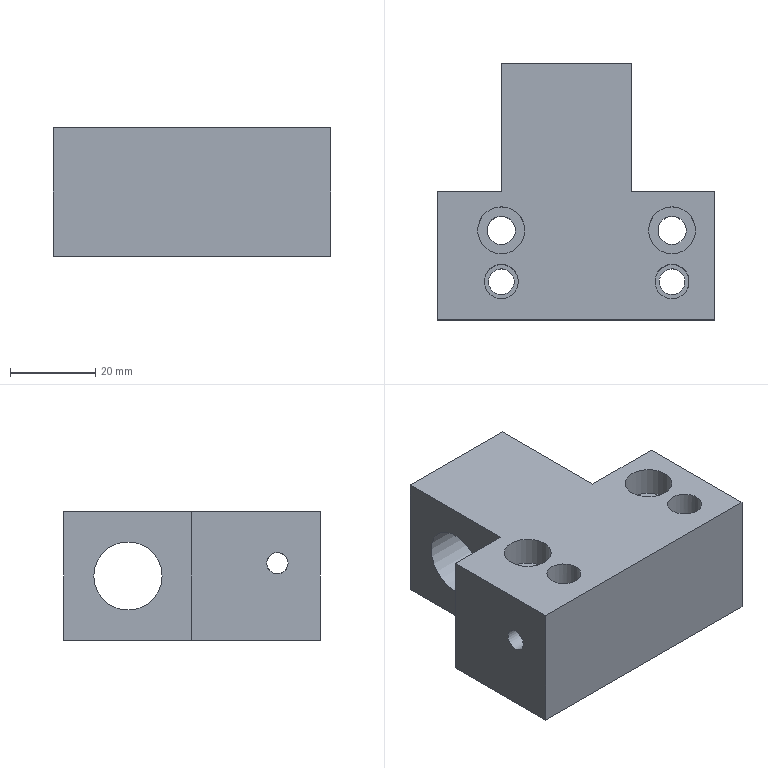Part | NX | features 5003_228_Bracket 2 | 1 solid | 26 faces | box 65 x 60 x 30 mm | volume 73363 mm3 | plane 14 | cylinder 12 | commonest cylinder face diameters 5 x3 6 x2 6.6 x2 8 x2 11 x2 16 x1
STEP:
#1=CARTESIAN_POINT('',(44.6,-182.,-208.));
#2=VERTEX_POINT('',#1);
#3=CARTESIAN_POINT('',(109.6,-182.,-208.));
#4=VERTEX_POINT('',#3);
#5=CARTESIAN_POINT('',(44.6,-182.,-208.));
#6=DIRECTION('',(1.,0.,0.));
#7=VECTOR('',#6,1000.);
#8=LINE('',#5,#7);
#9=EDGE_CURVE('',#2,#4,#8,.T.);
#10=ORIENTED_EDGE('',*,*,#9,.F.);
#11=CARTESIAN_POINT('',(44.6,-182.,-238.));
#12=VERTEX_POINT('',#11);
#13=CARTESIAN_POINT('',(44.6,-182.,-238.));
#14=DIRECTION('',(0.,0.,1.));
#15=VECTOR('',#14,1000.);
#16=LINE('',#13,#15);
#17=EDGE_CURVE('',#12,#2,#16,.T.);
#18=ORIENTED_EDGE('',*,*,#17,.F.);
#19=CARTESIAN_POINT('',(109.6,-182.,-238.));
#20=VERTEX_POINT('',#19);
#21=CARTESIAN_POINT('',(44.6,-182.,-238.));
#22=DIRECTION('',(1.,0.,0.));
#23=VECTOR('',#22,1000.);
#24=LINE('',#21,#23);
#25=EDGE_CURVE('',#12,#20,#24,.T.);
#26=ORIENTED_EDGE('',*,*,#25,.T.);
#27=CARTESIAN_POINT('',(109.6,-182.,-238.));
#28=DIRECTION('',(0.,0.,1.));
#29=VECTOR('',#28,1000.);
#30=LINE('',#27,#29);
#31=EDGE_CURVE('',#20,#4,#30,.T.);
#32=ORIENTED_EDGE('',*,*,#31,.T.);
#33=EDGE_LOOP('',(#10,#18,#26,#32));
#34=FACE_BOUND('',#33,.T.);
#35=CARTESIAN_POINT('',(44.6,-182.,-238.));
#36=DIRECTION('',(0.,-1.,0.));
#37=DIRECTION('',(1.,0.,0.));
#38=AXIS2_PLACEMENT_3D('',#35,#36,#37);
#39=PLANE('',#38);
#40=ADVANCED_FACE('',(#34),#39,.T.);
#41=CARTESIAN_POINT('',(44.6,-174.5,-220.));
#42=VERTEX_POINT('',#41);
#43=CARTESIAN_POINT('',(44.6,-172.,-220.));
#44=DIRECTION('',(-1.,0.,0.));
#45=DIRECTION('',(0.,-1.,0.));
#46=AXIS2_PLACEMENT_3D('',#43,#44,#45);
#47=CIRCLE('',#46,2.5);
#48=EDGE_CURVE('',#42,#42,#47,.T.);
#49=ORIENTED_EDGE('',*,*,#48,.F.);
#50=EDGE_LOOP('',(#49));
#51=FACE_BOUND('',#50,.T.);
#52=CARTESIAN_POINT('',(44.6,-152.,-208.));
#53=VERTEX_POINT('',#52);
#54=CARTESIAN_POINT('',(44.6,-152.,-238.));
#55=VERTEX_POINT('',#54);
#56=CARTESIAN_POINT('',(44.6,-152.,-208.));
#57=DIRECTION('',(0.,0.,-1.));
#58=VECTOR('',#57,1000.);
#59=LINE('',#56,#58);
#60=EDGE_CURVE('',#53,#55,#59,.T.);
#61=ORIENTED_EDGE('',*,*,#60,.T.);
#62=CARTESIAN_POINT('',(44.6,-122.,-238.));
#63=DIRECTION('',(0.,-1.,0.));
#64=VECTOR('',#63,1000.);
#65=LINE('',#62,#64);
#66=EDGE_CURVE('',#55,#12,#65,.T.);
#67=ORIENTED_EDGE('',*,*,#66,.T.);
#68=ORIENTED_EDGE('',*,*,#17,.T.);
#69=CARTESIAN_POINT('',(44.6,-122.,-208.));
#70=DIRECTION('',(0.,-1.,0.));
#71=VECTOR('',#70,1000.);
#72=LINE('',#69,#71);
#73=EDGE_CURVE('',#53,#2,#72,.T.);
#74=ORIENTED_EDGE('',*,*,#73,.F.);
#75=EDGE_LOOP('',(#61,#67,#68,#74));
#76=FACE_BOUND('',#75,.T.);
#77=CARTESIAN_POINT('',(44.6,-122.,-238.));
#78=DIRECTION('',(-1.,0.,0.));
#79=DIRECTION('',(0.,-1.,0.));
#80=AXIS2_PLACEMENT_3D('',#77,#78,#79);
#81=PLANE('',#80);
#82=ADVANCED_FACE('',(#51,#76),#81,.T.);
#83=CARTESIAN_POINT('',(90.089,-122.,-208.));
#84=VERTEX_POINT('',#83);
#85=CARTESIAN_POINT('',(90.089,-122.,-238.));
#86=VERTEX_POINT('',#85);
#87=CARTESIAN_POINT('',(90.089,-122.,-208.));
#88=DIRECTION('',(0.,0.,-1.));
#89=VECTOR('',#88,1000.);
#90=LINE('',#87,#89);
#91=EDGE_CURVE('',#84,#86,#90,.T.);
#92=ORIENTED_EDGE('',*,*,#91,.T.);
#93=CARTESIAN_POINT('',(59.6,-122.,-238.));
#94=VERTEX_POINT('',#93);
#95=CARTESIAN_POINT('',(109.6,-122.,-238.));
#96=DIRECTION('',(-1.,0.,0.));
#97=VECTOR('',#96,1000.);
#98=LINE('',#95,#97);
#99=EDGE_CURVE('',#86,#94,#98,.T.);
#100=ORIENTED_EDGE('',*,*,#99,.T.);
#101=CARTESIAN_POINT('',(59.6,-122.,-208.));
#102=VERTEX_POINT('',#101);
#103=CARTESIAN_POINT('',(59.6,-122.,-208.));
#104=DIRECTION('',(0.,0.,-1.));
#105=VECTOR('',#104,1000.);
#106=LINE('',#103,#105);
#107=EDGE_CURVE('',#102,#94,#106,.T.);
#108=ORIENTED_EDGE('',*,*,#107,.F.);
#109=CARTESIAN_POINT('',(109.6,-122.,-208.));
#110=DIRECTION('',(-1.,0.,0.));
#111=VECTOR('',#110,1000.);
#112=LINE('',#109,#111);
#113=EDGE_CURVE('',#84,#102,#112,.T.);
#114=ORIENTED_EDGE('',*,*,#113,.F.);
#115=EDGE_LOOP('',(#92,#100,#108,#114));
#116=FACE_BOUND('',#115,.T.);
#117=CARTESIAN_POINT('',(109.6,-122.,-238.));
#118=DIRECTION('',(0.,1.,0.));
#119=DIRECTION('',(-1.,0.,0.));
#120=AXIS2_PLACEMENT_3D('',#117,#118,#119);
#121=PLANE('',#120);
#122=ADVANCED_FACE('',(#116),#121,.T.);
#123=CARTESIAN_POINT('',(109.6,-169.5,-220.));
#124=VERTEX_POINT('',#123);
#125=CARTESIAN_POINT('',(109.6,-172.,-220.));
#126=DIRECTION('',(1.,0.,0.));
#127=DIRECTION('',(0.,1.,0.));
#128=AXIS2_PLACEMENT_3D('',#125,#126,#127);
#129=CIRCLE('',#128,2.5);
#130=EDGE_CURVE('',#124,#124,#129,.T.);
#131=ORIENTED_EDGE('',*,*,#130,.F.);
#132=EDGE_LOOP('',(#131));
#133=FACE_BOUND('',#132,.T.);
#134=CARTESIAN_POINT('',(109.6,-152.,-208.));
#135=VERTEX_POINT('',#134);
#136=CARTESIAN_POINT('',(109.6,-152.,-238.));
#137=VERTEX_POINT('',#136);
#138=CARTESIAN_POINT('',(109.6,-152.,-208.));
#139=DIRECTION('',(0.,0.,-1.));
#140=VECTOR('',#139,1000.);
#141=LINE('',#138,#140);
#142=EDGE_CURVE('',#135,#137,#141,.T.);
#143=ORIENTED_EDGE('',*,*,#142,.F.);
#144=CARTESIAN_POINT('',(109.6,-182.,-208.));
#145=DIRECTION('',(0.,1.,0.));
#146=VECTOR('',#145,1000.);
#147=LINE('',#144,#146);
#148=EDGE_CURVE('',#4,#135,#147,.T.);
#149=ORIENTED_EDGE('',*,*,#148,.F.);
#150=ORIENTED_EDGE('',*,*,#31,.F.);
#151=CARTESIAN_POINT('',(109.6,-182.,-238.));
#152=DIRECTION('',(0.,1.,0.));
#153=VECTOR('',#152,1000.);
#154=LINE('',#151,#153);
#155=EDGE_CURVE('',#20,#137,#154,.T.);
#156=ORIENTED_EDGE('',*,*,#155,.T.);
#157=EDGE_LOOP('',(#143,#149,#150,#156));
#158=FACE_BOUND('',#157,.T.);
#159=CARTESIAN_POINT('',(109.6,-182.,-238.));
#160=DIRECTION('',(1.,0.,0.));
#161=DIRECTION('',(0.,1.,0.));
#162=AXIS2_PLACEMENT_3D('',#159,#160,#161);
#163=PLANE('',#162);
#164=ADVANCED_FACE('',(#133,#158),#163,.T.);
#165=CARTESIAN_POINT('',(99.6,-176.,-238.));
#166=VERTEX_POINT('',#165);
#167=CARTESIAN_POINT('',(99.6,-173.,-238.));
#168=DIRECTION('',(0.,0.,1.));
#169=DIRECTION('',(0.,-1.,0.));
#170=AXIS2_PLACEMENT_3D('',#167,#168,#169);
#171=CIRCLE('',#170,3.);
#172=EDGE_CURVE('',#166,#166,#171,.T.);
#173=ORIENTED_EDGE('',*,*,#172,.T.);
#174=EDGE_LOOP('',(#173));
#175=FACE_BOUND('',#174,.T.);
#176=CARTESIAN_POINT('',(59.6,-176.,-238.));
#177=VERTEX_POINT('',#176);
#178=CARTESIAN_POINT('',(59.6,-173.,-238.));
#179=DIRECTION('',(0.,0.,1.));
#180=DIRECTION('',(0.,-1.,0.));
#181=AXIS2_PLACEMENT_3D('',#178,#179,#180);
#182=CIRCLE('',#181,3.);
#183=EDGE_CURVE('',#177,#177,#182,.T.);
#184=ORIENTED_EDGE('',*,*,#183,.T.);
#185=EDGE_LOOP('',(#184));
#186=FACE_BOUND('',#185,.T.);
#187=CARTESIAN_POINT('',(59.6,-164.3,-238.));
#188=VERTEX_POINT('',#187);
#189=CARTESIAN_POINT('',(59.6,-161.,-238.));
#190=DIRECTION('',(0.,0.,1.));
#191=DIRECTION('',(0.,-1.,0.));
#192=AXIS2_PLACEMENT_3D('',#189,#190,#191);
#193=CIRCLE('',#192,3.3);
#194=EDGE_CURVE('',#188,#188,#193,.T.);
#195=ORIENTED_EDGE('',*,*,#194,.T.);
#196=EDGE_LOOP('',(#195));
#197=FACE_BOUND('',#196,.T.);
#198=CARTESIAN_POINT('',(99.6,-164.3,-238.));
#199=VERTEX_POINT('',#198);
#200=CARTESIAN_POINT('',(99.6,-161.,-238.));
#201=DIRECTION('',(0.,0.,1.));
#202=DIRECTION('',(0.,-1.,0.));
#203=AXIS2_PLACEMENT_3D('',#200,#201,#202);
#204=CIRCLE('',#203,3.3);
#205=EDGE_CURVE('',#199,#199,#204,.T.);
#206=ORIENTED_EDGE('',*,*,#205,.T.);
#207=EDGE_LOOP('',(#206));
#208=FACE_BOUND('',#207,.T.);
#209=ORIENTED_EDGE('',*,*,#99,.F.);
#210=CARTESIAN_POINT('',(90.089,-152.,-238.));
#211=VERTEX_POINT('',#210);
#212=CARTESIAN_POINT('',(90.089,-152.,-238.));
#213=DIRECTION('',(0.,1.,0.));
#214=VECTOR('',#213,1000.);
#215=LINE('',#212,#214);
#216=EDGE_CURVE('',#211,#86,#215,.T.);
#217=ORIENTED_EDGE('',*,*,#216,.F.);
#218=CARTESIAN_POINT('',(109.6,-152.,-238.));
#219=DIRECTION('',(-1.,0.,0.));
#220=VECTOR('',#219,1000.);
#221=LINE('',#218,#220);
#222=EDGE_CURVE('',#137,#211,#221,.T.);
#223=ORIENTED_EDGE('',*,*,#222,.F.);
#224=ORIENTED_EDGE('',*,*,#155,.F.);
#225=ORIENTED_EDGE('',*,*,#25,.F.);
#226=ORIENTED_EDGE('',*,*,#66,.F.);
#227=CARTESIAN_POINT('',(59.6,-152.,-238.));
#228=VERTEX_POINT('',#227);
#229=CARTESIAN_POINT('',(59.6,-152.,-238.));
#230=DIRECTION('',(-1.,0.,0.));
#231=VECTOR('',#230,1000.);
#232=LINE('',#229,#231);
#233=EDGE_CURVE('',#228,#55,#232,.T.);
#234=ORIENTED_EDGE('',*,*,#233,.F.);
#235=CARTESIAN_POINT('',(59.6,-122.,-238.));
#236=DIRECTION('',(0.,-1.,0.));
#237=VECTOR('',#236,1000.);
#238=LINE('',#235,#237);
#239=EDGE_CURVE('',#94,#228,#238,.T.);
#240=ORIENTED_EDGE('',*,*,#239,.F.);
#241=EDGE_LOOP('',(#209,#217,#223,#224,#225,#226,#234,#240));
#242=FACE_BOUND('',#241,.T.);
#243=CARTESIAN_POINT('',(114.6,-182.,-238.));
#244=DIRECTION('',(0.,0.,1.));
#245=DIRECTION('',(0.,-1.,0.));
#246=AXIS2_PLACEMENT_3D('',#243,#244,#245);
#247=PLANE('',#246);
#248=ADVANCED_FACE('',(#175,#186,#197,#208,#242),#247,.F.);
#249=CARTESIAN_POINT('',(99.6,-177.,-208.));
#250=VERTEX_POINT('',#249);
#251=CARTESIAN_POINT('',(99.6,-173.,-208.));
#252=DIRECTION('',(0.,0.,1.));
#253=DIRECTION('',(0.,-1.,0.));
#254=AXIS2_PLACEMENT_3D('',#251,#252,#253);
#255=CIRCLE('',#254,4.);
#256=EDGE_CURVE('',#250,#250,#255,.T.);
#257=ORIENTED_EDGE('',*,*,#256,.F.);
#258=EDGE_LOOP('',(#257));
#259=FACE_BOUND('',#258,.T.);
#260=CARTESIAN_POINT('',(59.6,-177.,-208.));
#261=VERTEX_POINT('',#260);
#262=CARTESIAN_POINT('',(59.6,-173.,-208.));
#263=DIRECTION('',(0.,0.,1.));
#264=DIRECTION('',(0.,-1.,0.));
#265=AXIS2_PLACEMENT_3D('',#262,#263,#264);
#266=CIRCLE('',#265,4.);
#267=EDGE_CURVE('',#261,#261,#266,.T.);
#268=ORIENTED_EDGE('',*,*,#267,.F.);
#269=EDGE_LOOP('',(#268));
#270=FACE_BOUND('',#269,.T.);
#271=CARTESIAN_POINT('',(59.6,-166.5,-208.));
#272=VERTEX_POINT('',#271);
#273=CARTESIAN_POINT('',(59.6,-161.,-208.));
#274=DIRECTION('',(0.,0.,1.));
#275=DIRECTION('',(0.,-1.,0.));
#276=AXIS2_PLACEMENT_3D('',#273,#274,#275);
#277=CIRCLE('',#276,5.5);
#278=EDGE_CURVE('',#272,#272,#277,.T.);
#279=ORIENTED_EDGE('',*,*,#278,.F.);
#280=EDGE_LOOP('',(#279));
#281=FACE_BOUND('',#280,.T.);
#282=CARTESIAN_POINT('',(99.6,-166.5,-208.));
#283=VERTEX_POINT('',#282);
#284=CARTESIAN_POINT('',(99.6,-161.,-208.));
#285=DIRECTION('',(0.,0.,1.));
#286=DIRECTION('',(0.,-1.,0.));
#287=AXIS2_PLACEMENT_3D('',#284,#285,#286);
#288=CIRCLE('',#287,5.5);
#289=EDGE_CURVE('',#283,#283,#288,.T.);
#290=ORIENTED_EDGE('',*,*,#289,.F.);
#291=EDGE_LOOP('',(#290));
#292=FACE_BOUND('',#291,.T.);
#293=CARTESIAN_POINT('',(90.089,-152.,-208.));
#294=VERTEX_POINT('',#293);
#295=CARTESIAN_POINT('',(90.089,-152.,-208.));
#296=DIRECTION('',(0.,1.,0.));
#297=VECTOR('',#296,1000.);
#298=LINE('',#295,#297);
#299=EDGE_CURVE('',#294,#84,#298,.T.);
#300=ORIENTED_EDGE('',*,*,#299,.T.);
#301=ORIENTED_EDGE('',*,*,#113,.T.);
#302=CARTESIAN_POINT('',(59.6,-152.,-208.));
#303=VERTEX_POINT('',#302);
#304=CARTESIAN_POINT('',(59.6,-122.,-208.));
#305=DIRECTION('',(0.,-1.,0.));
#306=VECTOR('',#305,1000.);
#307=LINE('',#304,#306);
#308=EDGE_CURVE('',#102,#303,#307,.T.);
#309=ORIENTED_EDGE('',*,*,#308,.T.);
#310=CARTESIAN_POINT('',(59.6,-152.,-208.));
#311=DIRECTION('',(-1.,0.,0.));
#312=VECTOR('',#311,1000.);
#313=LINE('',#310,#312);
#314=EDGE_CURVE('',#303,#53,#313,.T.);
#315=ORIENTED_EDGE('',*,*,#314,.T.);
#316=ORIENTED_EDGE('',*,*,#73,.T.);
#317=ORIENTED_EDGE('',*,*,#9,.T.);
#318=ORIENTED_EDGE('',*,*,#148,.T.);
#319=CARTESIAN_POINT('',(109.6,-152.,-208.));
#320=DIRECTION('',(-1.,0.,0.));
#321=VECTOR('',#320,1000.);
#322=LINE('',#319,#321);
#323=EDGE_CURVE('',#135,#294,#322,.T.);
#324=ORIENTED_EDGE('',*,*,#323,.T.);
#325=EDGE_LOOP('',(#300,#301,#309,#315,#316,#317,#318,#324));
#326=FACE_BOUND('',#325,.T.);
#327=CARTESIAN_POINT('',(114.6,-182.,-208.));
#328=DIRECTION('',(0.,0.,1.));
#329=DIRECTION('',(0.,-1.,0.));
#330=AXIS2_PLACEMENT_3D('',#327,#328,#329);
#331=PLANE('',#330);
#332=ADVANCED_FACE('',(#259,#270,#281,#292,#326),#331,.T.);
#333=ORIENTED_EDGE('',*,*,#233,.T.);
#334=ORIENTED_EDGE('',*,*,#60,.F.);
#335=ORIENTED_EDGE('',*,*,#314,.F.);
#336=CARTESIAN_POINT('',(59.6,-152.,-208.));
#337=DIRECTION('',(0.,0.,-1.));
#338=VECTOR('',#337,1000.);
#339=LINE('',#336,#338);
#340=EDGE_CURVE('',#303,#228,#339,.T.);
#341=ORIENTED_EDGE('',*,*,#340,.T.);
#342=EDGE_LOOP('',(#333,#334,#335,#341));
#343=FACE_BOUND('',#342,.T.);
#344=CARTESIAN_POINT('',(59.6,-152.,-208.));
#345=DIRECTION('',(0.,-1.,0.));
#346=DIRECTION('',(1.,0.,0.));
#347=AXIS2_PLACEMENT_3D('',#344,#345,#346);
#348=PLANE('',#347);
#349=ADVANCED_FACE('',(#343),#348,.F.);
#350=CARTESIAN_POINT('',(59.6,-145.,-223.));
#351=VERTEX_POINT('',#350);
#352=CARTESIAN_POINT('',(59.6,-137.,-223.));
#353=DIRECTION('',(-1.,0.,0.));
#354=DIRECTION('',(0.,-1.,0.));
#355=AXIS2_PLACEMENT_3D('',#352,#353,#354);
#356=CIRCLE('',#355,8.);
#357=EDGE_CURVE('',#351,#351,#356,.T.);
#358=ORIENTED_EDGE('',*,*,#357,.F.);
#359=EDGE_LOOP('',(#358));
#360=FACE_BOUND('',#359,.T.);
#361=ORIENTED_EDGE('',*,*,#239,.T.);
#362=ORIENTED_EDGE('',*,*,#340,.F.);
#363=ORIENTED_EDGE('',*,*,#308,.F.);
#364=ORIENTED_EDGE('',*,*,#107,.T.);
#365=EDGE_LOOP('',(#361,#362,#363,#364));
#366=FACE_BOUND('',#365,.T.);
#367=CARTESIAN_POINT('',(59.6,-122.,-208.));
#368=DIRECTION('',(1.,0.,0.));
#369=DIRECTION('',(0.,1.,0.));
#370=AXIS2_PLACEMENT_3D('',#367,#368,#369);
#371=PLANE('',#370);
#372=ADVANCED_FACE('',(#360,#366),#371,.F.);
#373=CARTESIAN_POINT('',(90.089,-145.,-223.));
#374=VERTEX_POINT('',#373);
#375=CARTESIAN_POINT('',(90.089,-137.,-223.));
#376=DIRECTION('',(-1.,0.,0.));
#377=DIRECTION('',(0.,-1.,0.));
#378=AXIS2_PLACEMENT_3D('',#375,#376,#377);
#379=CIRCLE('',#378,8.);
#380=EDGE_CURVE('',#374,#374,#379,.T.);
#381=ORIENTED_EDGE('',*,*,#380,.T.);
#382=EDGE_LOOP('',(#381));
#383=FACE_BOUND('',#382,.T.);
#384=ORIENTED_EDGE('',*,*,#216,.T.);
#385=ORIENTED_EDGE('',*,*,#91,.F.);
#386=ORIENTED_EDGE('',*,*,#299,.F.);
#387=CARTESIAN_POINT('',(90.089,-152.,-208.));
#388=DIRECTION('',(0.,0.,-1.));
#389=VECTOR('',#388,1000.);
#390=LINE('',#387,#389);
#391=EDGE_CURVE('',#294,#211,#390,.T.);
#392=ORIENTED_EDGE('',*,*,#391,.T.);
#393=EDGE_LOOP('',(#384,#385,#386,#392));
#394=FACE_BOUND('',#393,.T.);
#395=CARTESIAN_POINT('',(90.089,-152.,-208.));
#396=DIRECTION('',(-1.,0.,0.));
#397=DIRECTION('',(0.,-1.,0.));
#398=AXIS2_PLACEMENT_3D('',#395,#396,#397);
#399=PLANE('',#398);
#400=ADVANCED_FACE('',(#383,#394),#399,.F.);
#401=ORIENTED_EDGE('',*,*,#222,.T.);
#402=ORIENTED_EDGE('',*,*,#391,.F.);
#403=ORIENTED_EDGE('',*,*,#323,.F.);
#404=ORIENTED_EDGE('',*,*,#142,.T.);
#405=EDGE_LOOP('',(#401,#402,#403,#404));
#406=FACE_BOUND('',#405,.T.);
#407=CARTESIAN_POINT('',(109.6,-152.,-208.));
#408=DIRECTION('',(0.,-1.,0.));
#409=DIRECTION('',(1.,0.,0.));
#410=AXIS2_PLACEMENT_3D('',#407,#408,#409);
#411=PLANE('',#410);
#412=ADVANCED_FACE('',(#406),#411,.F.);
#413=ORIENTED_EDGE('',*,*,#357,.T.);
#414=EDGE_LOOP('',(#413));
#415=FACE_BOUND('',#414,.T.);
#416=ORIENTED_EDGE('',*,*,#380,.F.);
#417=EDGE_LOOP('',(#416));
#418=FACE_BOUND('',#417,.T.);
#419=CARTESIAN_POINT('',(59.6,-137.,-223.));
#420=DIRECTION('',(-1.,0.,0.));
#421=DIRECTION('',(0.,-1.,0.));
#422=AXIS2_PLACEMENT_3D('',#419,#420,#421);
#423=CYLINDRICAL_SURFACE('',#422,8.);
#424=ADVANCED_FACE('',(#415,#418),#423,.F.);
#425=ORIENTED_EDGE('',*,*,#205,.F.);
#426=EDGE_LOOP('',(#425));
#427=FACE_BOUND('',#426,.T.);
#428=CARTESIAN_POINT('',(99.6,-164.3,-214.8));
#429=VERTEX_POINT('',#428);
#430=CARTESIAN_POINT('',(99.6,-161.,-214.8));
#431=DIRECTION('',(0.,0.,1.));
#432=DIRECTION('',(0.,-1.,0.));
#433=AXIS2_PLACEMENT_3D('',#430,#431,#432);
#434=CIRCLE('',#433,3.3);
#435=EDGE_CURVE('',#429,#429,#434,.T.);
#436=ORIENTED_EDGE('',*,*,#435,.T.);
#437=EDGE_LOOP('',(#436));
#438=FACE_BOUND('',#437,.T.);
#439=CARTESIAN_POINT('',(99.6,-161.,-208.));
#440=DIRECTION('',(0.,0.,1.));
#441=DIRECTION('',(0.,-1.,0.));
#442=AXIS2_PLACEMENT_3D('',#439,#440,#441);
#443=CYLINDRICAL_SURFACE('',#442,3.3);
#444=ADVANCED_FACE('',(#427,#438),#443,.F.);
#445=ORIENTED_EDGE('',*,*,#435,.F.);
#446=EDGE_LOOP('',(#445));
#447=FACE_BOUND('',#446,.T.);
#448=CARTESIAN_POINT('',(99.6,-166.5,-214.8));
#449=VERTEX_POINT('',#448);
#450=CARTESIAN_POINT('',(99.6,-161.,-214.8));
#451=DIRECTION('',(0.,0.,1.));
#452=DIRECTION('',(0.,-1.,0.));
#453=AXIS2_PLACEMENT_3D('',#450,#451,#452);
#454=CIRCLE('',#453,5.5);
#455=EDGE_CURVE('',#449,#449,#454,.T.);
#456=ORIENTED_EDGE('',*,*,#455,.T.);
#457=EDGE_LOOP('',(#456));
#458=FACE_BOUND('',#457,.T.);
#459=CARTESIAN_POINT('',(102.9,-161.,-214.8));
#460=DIRECTION('',(0.,0.,-1.));
#461=DIRECTION('',(0.,1.,0.));
#462=AXIS2_PLACEMENT_3D('',#459,#460,#461);
#463=PLANE('',#462);
#464=ADVANCED_FACE('',(#447,#458),#463,.F.);
#465=ORIENTED_EDGE('',*,*,#455,.F.);
#466=EDGE_LOOP('',(#465));
#467=FACE_BOUND('',#466,.T.);
#468=ORIENTED_EDGE('',*,*,#289,.T.);
#469=EDGE_LOOP('',(#468));
#470=FACE_BOUND('',#469,.T.);
#471=CARTESIAN_POINT('',(99.6,-161.,-208.));
#472=DIRECTION('',(0.,0.,1.));
#473=DIRECTION('',(0.,-1.,0.));
#474=AXIS2_PLACEMENT_3D('',#471,#472,#473);
#475=CYLINDRICAL_SURFACE('',#474,5.5);
#476=ADVANCED_FACE('',(#467,#470),#475,.F.);
#477=ORIENTED_EDGE('',*,*,#194,.F.);
#478=EDGE_LOOP('',(#477));
#479=FACE_BOUND('',#478,.T.);
#480=CARTESIAN_POINT('',(59.6,-164.3,-214.8));
#481=VERTEX_POINT('',#480);
#482=CARTESIAN_POINT('',(59.6,-161.,-214.8));
#483=DIRECTION('',(0.,0.,1.));
#484=DIRECTION('',(0.,-1.,0.));
#485=AXIS2_PLACEMENT_3D('',#482,#483,#484);
#486=CIRCLE('',#485,3.3);
#487=EDGE_CURVE('',#481,#481,#486,.T.);
#488=ORIENTED_EDGE('',*,*,#487,.T.);
#489=EDGE_LOOP('',(#488));
#490=FACE_BOUND('',#489,.T.);
#491=CARTESIAN_POINT('',(59.6,-161.,-208.));
#492=DIRECTION('',(0.,0.,1.));
#493=DIRECTION('',(0.,-1.,0.));
#494=AXIS2_PLACEMENT_3D('',#491,#492,#493);
#495=CYLINDRICAL_SURFACE('',#494,3.3);
#496=ADVANCED_FACE('',(#479,#490),#495,.F.);
#497=ORIENTED_EDGE('',*,*,#487,.F.);
#498=EDGE_LOOP('',(#497));
#499=FACE_BOUND('',#498,.T.);
#500=CARTESIAN_POINT('',(59.6,-166.5,-214.8));
#501=VERTEX_POINT('',#500);
#502=CARTESIAN_POINT('',(59.6,-161.,-214.8));
#503=DIRECTION('',(0.,0.,1.));
#504=DIRECTION('',(0.,-1.,0.));
#505=AXIS2_PLACEMENT_3D('',#502,#503,#504);
#506=CIRCLE('',#505,5.5);
#507=EDGE_CURVE('',#501,#501,#506,.T.);
#508=ORIENTED_EDGE('',*,*,#507,.T.);
#509=EDGE_LOOP('',(#508));
#510=FACE_BOUND('',#509,.T.);
#511=CARTESIAN_POINT('',(62.9,-161.,-214.8));
#512=DIRECTION('',(0.,0.,-1.));
#513=DIRECTION('',(0.,1.,0.));
#514=AXIS2_PLACEMENT_3D('',#511,#512,#513);
#515=PLANE('',#514);
#516=ADVANCED_FACE('',(#499,#510),#515,.F.);
#517=ORIENTED_EDGE('',*,*,#507,.F.);
#518=EDGE_LOOP('',(#517));
#519=FACE_BOUND('',#518,.T.);
#520=ORIENTED_EDGE('',*,*,#278,.T.);
#521=EDGE_LOOP('',(#520));
#522=FACE_BOUND('',#521,.T.);
#523=CARTESIAN_POINT('',(59.6,-161.,-208.));
#524=DIRECTION('',(0.,0.,1.));
#525=DIRECTION('',(0.,-1.,0.));
#526=AXIS2_PLACEMENT_3D('',#523,#524,#525);
#527=CYLINDRICAL_SURFACE('',#526,5.5);
#528=ADVANCED_FACE('',(#519,#522),#527,.F.);
#529=ORIENTED_EDGE('',*,*,#183,.F.);
#530=EDGE_LOOP('',(#529));
#531=FACE_BOUND('',#530,.T.);
#532=CARTESIAN_POINT('',(59.6,-176.,-228.));
#533=VERTEX_POINT('',#532);
#534=CARTESIAN_POINT('',(59.6,-173.,-228.));
#535=DIRECTION('',(0.,0.,1.));
#536=DIRECTION('',(0.,-1.,0.));
#537=AXIS2_PLACEMENT_3D('',#534,#535,#536);
#538=CIRCLE('',#537,3.);
#539=EDGE_CURVE('',#533,#533,#538,.T.);
#540=ORIENTED_EDGE('',*,*,#539,.T.);
#541=EDGE_LOOP('',(#540));
#542=FACE_BOUND('',#541,.T.);
#543=CARTESIAN_POINT('',(59.6,-173.,-208.));
#544=DIRECTION('',(0.,0.,1.));
#545=DIRECTION('',(0.,-1.,0.));
#546=AXIS2_PLACEMENT_3D('',#543,#544,#545);
#547=CYLINDRICAL_SURFACE('',#546,3.);
#548=ADVANCED_FACE('',(#531,#542),#547,.F.);
#549=ORIENTED_EDGE('',*,*,#539,.F.);
#550=EDGE_LOOP('',(#549));
#551=FACE_BOUND('',#550,.T.);
#552=CARTESIAN_POINT('',(59.6,-177.,-228.));
#553=VERTEX_POINT('',#552);
#554=CARTESIAN_POINT('',(59.6,-173.,-228.));
#555=DIRECTION('',(0.,0.,1.));
#556=DIRECTION('',(0.,-1.,0.));
#557=AXIS2_PLACEMENT_3D('',#554,#555,#556);
#558=CIRCLE('',#557,4.);
#559=EDGE_CURVE('',#553,#553,#558,.T.);
#560=ORIENTED_EDGE('',*,*,#559,.T.);
#561=EDGE_LOOP('',(#560));
#562=FACE_BOUND('',#561,.T.);
#563=CARTESIAN_POINT('',(62.6,-173.,-228.));
#564=DIRECTION('',(0.,0.,-1.));
#565=DIRECTION('',(0.,1.,0.));
#566=AXIS2_PLACEMENT_3D('',#563,#564,#565);
#567=PLANE('',#566);
#568=ADVANCED_FACE('',(#551,#562),#567,.F.);
#569=CARTESIAN_POINT('',(63.309,-174.5,-220.));
#570=VERTEX_POINT('',#569);
#571=CARTESIAN_POINT('',(63.529,-174.044,-218.277));
#572=CARTESIAN_POINT('',(63.162,-174.804,-220.));
#573=CARTESIAN_POINT('',(63.529,-174.043,-221.722));
#574=CARTESIAN_POINT('',(63.64,-172.816,-222.442));
#575=CARTESIAN_POINT('',(63.452,-171.755,-222.557));
#576=CARTESIAN_POINT('',(63.005,-170.827,-222.271));
#577=CARTESIAN_POINT('',(62.427,-170.128,-221.725));
#578=CARTESIAN_POINT('',(61.821,-169.652,-221.014));
#579=CARTESIAN_POINT('',(61.395,-169.424,-219.999));
#580=CARTESIAN_POINT('',(61.823,-169.653,-218.984));
#581=CARTESIAN_POINT('',(62.426,-170.128,-218.275));
#582=CARTESIAN_POINT('',(63.002,-170.823,-217.732));
#583=CARTESIAN_POINT('',(63.45,-171.749,-217.444));
#584=CARTESIAN_POINT('',(63.64,-172.807,-217.555));
#585=CARTESIAN_POINT('',(63.529,-174.044,-218.277));
#586=CARTESIAN_POINT('',(63.162,-174.804,-220.));
#587=CARTESIAN_POINT('',(63.529,-174.043,-221.722));
#588=B_SPLINE_CURVE_WITH_KNOTS('',3,(#571,#572,#573,#574,#575,#576,#577,#578,#579,#580,#581,#582,#583,#584,#585,#586,#587),.UNSPECIFIED.,.T.,.F.,(1,1,1,1,1,1,1,1,1,1,1,1,1,1,1,1,1,1,1,1,1),(-0.004166,-0.003124,-0.002083,0.,0.002083,0.003124,0.004166,0.005207,0.006249,0.00729,0.008331,0.009373,0.01041,0.01146,0.0125,0.01354,0.01458,0.01666,0.01875,0.01979,0.02083),.UNSPECIFIED.);
#589=EDGE_CURVE('',#570,#570,#588,.T.);
#590=ORIENTED_EDGE('',*,*,#589,.T.);
#591=EDGE_LOOP('',(#590));
#592=FACE_BOUND('',#591,.T.);
#593=CARTESIAN_POINT('',(55.892,-174.5,-220.));
#594=VERTEX_POINT('',#593);
#595=CARTESIAN_POINT('',(55.672,-174.044,-221.723));
#596=CARTESIAN_POINT('',(56.039,-174.804,-220.));
#597=CARTESIAN_POINT('',(55.672,-174.043,-218.278));
#598=CARTESIAN_POINT('',(55.561,-172.816,-217.558));
#599=CARTESIAN_POINT('',(55.749,-171.755,-217.443));
#600=CARTESIAN_POINT('',(56.196,-170.827,-217.729));
#601=CARTESIAN_POINT('',(56.774,-170.128,-218.275));
#602=CARTESIAN_POINT('',(57.38,-169.652,-218.986));
#603=CARTESIAN_POINT('',(57.806,-169.424,-220.001));
#604=CARTESIAN_POINT('',(57.378,-169.653,-221.016));
#605=CARTESIAN_POINT('',(56.775,-170.128,-221.725));
#606=CARTESIAN_POINT('',(56.199,-170.823,-222.268));
#607=CARTESIAN_POINT('',(55.751,-171.749,-222.556));
#608=CARTESIAN_POINT('',(55.561,-172.807,-222.445));
#609=CARTESIAN_POINT('',(55.672,-174.044,-221.723));
#610=CARTESIAN_POINT('',(56.039,-174.804,-220.));
#611=CARTESIAN_POINT('',(55.672,-174.043,-218.278));
#612=B_SPLINE_CURVE_WITH_KNOTS('',3,(#595,#596,#597,#598,#599,#600,#601,#602,#603,#604,#605,#606,#607,#608,#609,#610,#611),.UNSPECIFIED.,.T.,.F.,(1,1,1,1,1,1,1,1,1,1,1,1,1,1,1,1,1,1,1,1,1),(-0.004166,-0.003124,-0.002083,0.,0.002083,0.003124,0.004166,0.005207,0.006249,0.00729,0.008331,0.009373,0.01041,0.01146,0.0125,0.01354,0.01458,0.01666,0.01875,0.01979,0.02083),.UNSPECIFIED.);
#613=EDGE_CURVE('',#594,#594,#612,.T.);
#614=ORIENTED_EDGE('',*,*,#613,.T.);
#615=EDGE_LOOP('',(#614));
#616=FACE_BOUND('',#615,.T.);
#617=ORIENTED_EDGE('',*,*,#559,.F.);
#618=EDGE_LOOP('',(#617));
#619=FACE_BOUND('',#618,.T.);
#620=ORIENTED_EDGE('',*,*,#267,.T.);
#621=EDGE_LOOP('',(#620));
#622=FACE_BOUND('',#621,.T.);
#623=CARTESIAN_POINT('',(59.6,-173.,-208.));
#624=DIRECTION('',(0.,0.,1.));
#625=DIRECTION('',(0.,-1.,0.));
#626=AXIS2_PLACEMENT_3D('',#623,#624,#625);
#627=CYLINDRICAL_SURFACE('',#626,4.);
#628=ADVANCED_FACE('',(#592,#616,#619,#622),#627,.F.);
#629=ORIENTED_EDGE('',*,*,#172,.F.);
#630=EDGE_LOOP('',(#629));
#631=FACE_BOUND('',#630,.T.);
#632=CARTESIAN_POINT('',(99.6,-176.,-228.));
#633=VERTEX_POINT('',#632);
#634=CARTESIAN_POINT('',(99.6,-173.,-228.));
#635=DIRECTION('',(0.,0.,1.));
#636=DIRECTION('',(0.,-1.,0.));
#637=AXIS2_PLACEMENT_3D('',#634,#635,#636);
#638=CIRCLE('',#637,3.);
#639=EDGE_CURVE('',#633,#633,#638,.T.);
#640=ORIENTED_EDGE('',*,*,#639,.T.);
#641=EDGE_LOOP('',(#640));
#642=FACE_BOUND('',#641,.T.);
#643=CARTESIAN_POINT('',(99.6,-173.,-208.));
#644=DIRECTION('',(0.,0.,1.));
#645=DIRECTION('',(0.,-1.,0.));
#646=AXIS2_PLACEMENT_3D('',#643,#644,#645);
#647=CYLINDRICAL_SURFACE('',#646,3.);
#648=ADVANCED_FACE('',(#631,#642),#647,.F.);
#649=ORIENTED_EDGE('',*,*,#639,.F.);
#650=EDGE_LOOP('',(#649));
#651=FACE_BOUND('',#650,.T.);
#652=CARTESIAN_POINT('',(99.6,-177.,-228.));
#653=VERTEX_POINT('',#652);
#654=CARTESIAN_POINT('',(99.6,-173.,-228.));
#655=DIRECTION('',(0.,0.,1.));
#656=DIRECTION('',(0.,-1.,0.));
#657=AXIS2_PLACEMENT_3D('',#654,#655,#656);
#658=CIRCLE('',#657,4.);
#659=EDGE_CURVE('',#653,#653,#658,.T.);
#660=ORIENTED_EDGE('',*,*,#659,.T.);
#661=EDGE_LOOP('',(#660));
#662=FACE_BOUND('',#661,.T.);
#663=CARTESIAN_POINT('',(102.6,-173.,-228.));
#664=DIRECTION('',(0.,0.,-1.));
#665=DIRECTION('',(0.,1.,0.));
#666=AXIS2_PLACEMENT_3D('',#663,#664,#665);
#667=PLANE('',#666);
#668=ADVANCED_FACE('',(#651,#662),#667,.F.);
#669=CARTESIAN_POINT('',(103.309,-174.5,-220.));
#670=VERTEX_POINT('',#669);
#671=CARTESIAN_POINT('',(103.529,-174.044,-218.277));
#672=CARTESIAN_POINT('',(103.162,-174.804,-220.));
#673=CARTESIAN_POINT('',(103.529,-174.043,-221.722));
#674=CARTESIAN_POINT('',(103.64,-172.816,-222.442));
#675=CARTESIAN_POINT('',(103.452,-171.755,-222.557));
#676=CARTESIAN_POINT('',(103.005,-170.827,-222.271));
#677=CARTESIAN_POINT('',(102.427,-170.128,-221.725));
#678=CARTESIAN_POINT('',(101.821,-169.652,-221.014));
#679=CARTESIAN_POINT('',(101.395,-169.424,-219.999));
#680=CARTESIAN_POINT('',(101.823,-169.653,-218.984));
#681=CARTESIAN_POINT('',(102.426,-170.128,-218.275));
#682=CARTESIAN_POINT('',(103.002,-170.823,-217.732));
#683=CARTESIAN_POINT('',(103.45,-171.749,-217.444));
#684=CARTESIAN_POINT('',(103.64,-172.807,-217.555));
#685=CARTESIAN_POINT('',(103.529,-174.044,-218.277));
#686=CARTESIAN_POINT('',(103.162,-174.804,-220.));
#687=CARTESIAN_POINT('',(103.529,-174.043,-221.722));
#688=B_SPLINE_CURVE_WITH_KNOTS('',3,(#671,#672,#673,#674,#675,#676,#677,#678,#679,#680,#681,#682,#683,#684,#685,#686,#687),.UNSPECIFIED.,.T.,.F.,(1,1,1,1,1,1,1,1,1,1,1,1,1,1,1,1,1,1,1,1,1),(-0.004166,-0.003124,-0.002083,0.,0.002083,0.003124,0.004166,0.005207,0.006249,0.00729,0.008331,0.009373,0.01041,0.01146,0.0125,0.01354,0.01458,0.01666,0.01875,0.01979,0.02083),.UNSPECIFIED.);
#689=EDGE_CURVE('',#670,#670,#688,.T.);
#690=ORIENTED_EDGE('',*,*,#689,.T.);
#691=EDGE_LOOP('',(#690));
#692=FACE_BOUND('',#691,.T.);
#693=CARTESIAN_POINT('',(95.892,-174.5,-220.));
#694=VERTEX_POINT('',#693);
#695=CARTESIAN_POINT('',(95.672,-174.044,-221.723));
#696=CARTESIAN_POINT('',(96.039,-174.804,-220.));
#697=CARTESIAN_POINT('',(95.672,-174.043,-218.278));
#698=CARTESIAN_POINT('',(95.561,-172.816,-217.558));
#699=CARTESIAN_POINT('',(95.749,-171.755,-217.443));
#700=CARTESIAN_POINT('',(96.196,-170.827,-217.729));
#701=CARTESIAN_POINT('',(96.774,-170.128,-218.275));
#702=CARTESIAN_POINT('',(97.38,-169.652,-218.986));
#703=CARTESIAN_POINT('',(97.806,-169.424,-220.001));
#704=CARTESIAN_POINT('',(97.378,-169.653,-221.016));
#705=CARTESIAN_POINT('',(96.775,-170.128,-221.725));
#706=CARTESIAN_POINT('',(96.199,-170.823,-222.268));
#707=CARTESIAN_POINT('',(95.751,-171.749,-222.556));
#708=CARTESIAN_POINT('',(95.561,-172.807,-222.445));
#709=CARTESIAN_POINT('',(95.672,-174.044,-221.723));
#710=CARTESIAN_POINT('',(96.039,-174.804,-220.));
#711=CARTESIAN_POINT('',(95.672,-174.043,-218.278));
#712=B_SPLINE_CURVE_WITH_KNOTS('',3,(#695,#696,#697,#698,#699,#700,#701,#702,#703,#704,#705,#706,#707,#708,#709,#710,#711),.UNSPECIFIED.,.T.,.F.,(1,1,1,1,1,1,1,1,1,1,1,1,1,1,1,1,1,1,1,1,1),(-0.004166,-0.003124,-0.002083,0.,0.002083,0.003124,0.004166,0.005207,0.006249,0.00729,0.008331,0.009373,0.01041,0.01146,0.0125,0.01354,0.01458,0.01666,0.01875,0.01979,0.02083),.UNSPECIFIED.);
#713=EDGE_CURVE('',#694,#694,#712,.T.);
#714=ORIENTED_EDGE('',*,*,#713,.T.);
#715=EDGE_LOOP('',(#714));
#716=FACE_BOUND('',#715,.T.);
#717=ORIENTED_EDGE('',*,*,#659,.F.);
#718=EDGE_LOOP('',(#717));
#719=FACE_BOUND('',#718,.T.);
#720=ORIENTED_EDGE('',*,*,#256,.T.);
#721=EDGE_LOOP('',(#720));
#722=FACE_BOUND('',#721,.T.);
#723=CARTESIAN_POINT('',(99.6,-173.,-208.));
#724=DIRECTION('',(0.,0.,1.));
#725=DIRECTION('',(0.,-1.,0.));
#726=AXIS2_PLACEMENT_3D('',#723,#724,#725);
#727=CYLINDRICAL_SURFACE('',#726,4.);
#728=ADVANCED_FACE('',(#692,#716,#719,#722),#727,.F.);
#729=ORIENTED_EDGE('',*,*,#48,.T.);
#730=EDGE_LOOP('',(#729));
#731=FACE_BOUND('',#730,.T.);
#732=ORIENTED_EDGE('',*,*,#613,.F.);
#733=EDGE_LOOP('',(#732));
#734=FACE_BOUND('',#733,.T.);
#735=CARTESIAN_POINT('',(44.6,-172.,-220.));
#736=DIRECTION('',(-1.,0.,0.));
#737=DIRECTION('',(0.,-1.,0.));
#738=AXIS2_PLACEMENT_3D('',#735,#736,#737);
#739=CYLINDRICAL_SURFACE('',#738,2.5);
#740=ADVANCED_FACE('',(#731,#734),#739,.F.);
#741=ORIENTED_EDGE('',*,*,#713,.F.);
#742=EDGE_LOOP('',(#741));
#743=FACE_BOUND('',#742,.T.);
#744=ORIENTED_EDGE('',*,*,#589,.F.);
#745=EDGE_LOOP('',(#744));
#746=FACE_BOUND('',#745,.T.);
#747=CARTESIAN_POINT('',(44.6,-172.,-220.));
#748=DIRECTION('',(-1.,0.,0.));
#749=DIRECTION('',(0.,-1.,0.));
#750=AXIS2_PLACEMENT_3D('',#747,#748,#749);
#751=CYLINDRICAL_SURFACE('',#750,2.5);
#752=ADVANCED_FACE('',(#743,#746),#751,.F.);
#753=ORIENTED_EDGE('',*,*,#130,.T.);
#754=EDGE_LOOP('',(#753));
#755=FACE_BOUND('',#754,.T.);
#756=ORIENTED_EDGE('',*,*,#689,.F.);
#757=EDGE_LOOP('',(#756));
#758=FACE_BOUND('',#757,.T.);
#759=CARTESIAN_POINT('',(44.6,-172.,-220.));
#760=DIRECTION('',(-1.,0.,0.));
#761=DIRECTION('',(0.,-1.,0.));
#762=AXIS2_PLACEMENT_3D('',#759,#760,#761);
#763=CYLINDRICAL_SURFACE('',#762,2.5);
#764=ADVANCED_FACE('',(#755,#758),#763,.F.);
#765=CLOSED_SHELL('',(#40,#82,#122,#164,#248,#332,#349,#372,#400,#412,#424,#444,#464,#476,#496,#516,#528,#548,#568,#628,#648,#668,#728,#740,#752,#764));
#766=MANIFOLD_SOLID_BREP('',#765);
#767=(LENGTH_UNIT()NAMED_UNIT(*)SI_UNIT(.MILLI.,.METRE.));
#768=UNCERTAINTY_MEASURE_WITH_UNIT(LENGTH_MEASURE(0.0508),#767,'','');
#769=(NAMED_UNIT(*)PLANE_ANGLE_UNIT()SI_UNIT($,.RADIAN.));
#770=(NAMED_UNIT(*)SI_UNIT($,.STERADIAN.)SOLID_ANGLE_UNIT());
#771=(GEOMETRIC_REPRESENTATION_CONTEXT(3)GLOBAL_UNCERTAINTY_ASSIGNED_CONTEXT((#768))GLOBAL_UNIT_ASSIGNED_CONTEXT((#767,#769,#770))REPRESENTATION_CONTEXT('',''));
#772=ADVANCED_BREP_SHAPE_REPRESENTATION('',(#766),#771);